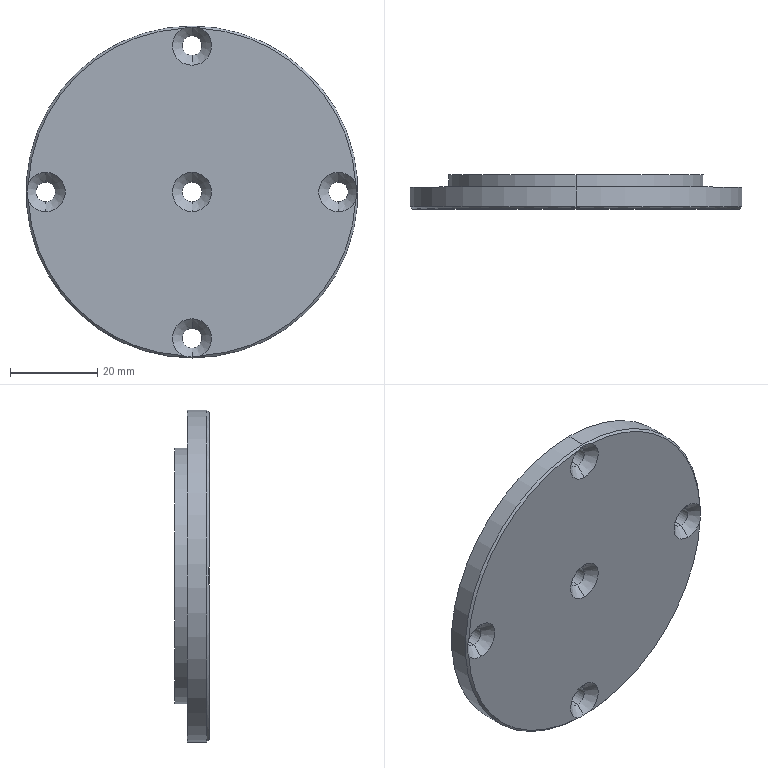Part | STEP file | ND25021-01-JDKM-41-TL | 1 solid | 34 faces | box 76 x 7.8 x 76 mm | volume 28044 mm3 | cylinder 16 | cone 14 | plane 4 | commonest cylinder face diameters 4.5 x10 25.2 x2 58.5 x2 76 x2